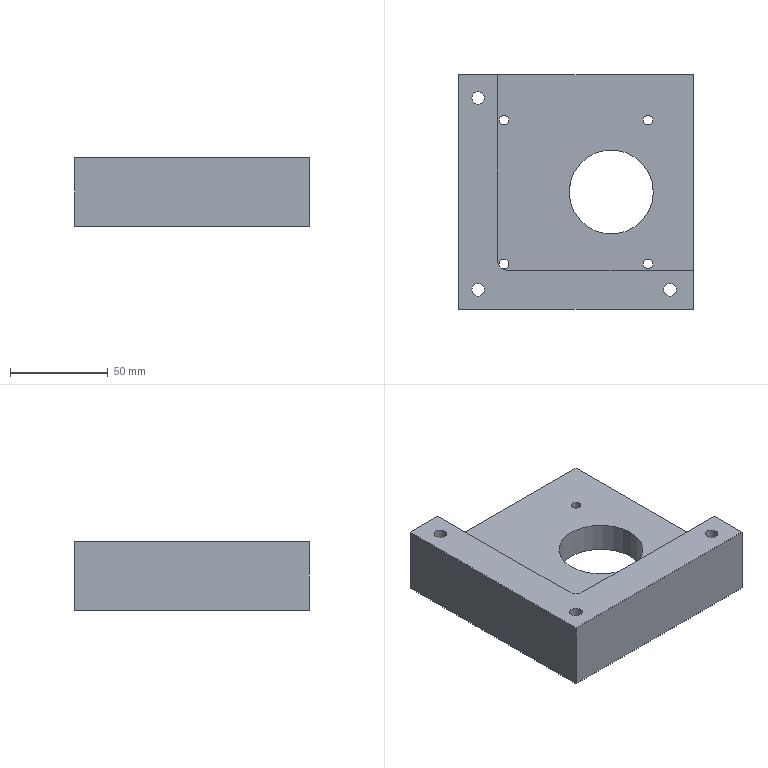Part | NX | 1 solid | 24 faces | box 120 x 120 x 35 mm | volume 274066 mm3 | plane 12 | cylinder 12 | commonest cylinder face diameters 5 x4 6.5 x3 12 x3 10 x1 43 x1
STEP:
#1=CARTESIAN_POINT('',(-60.,60.,-17.5));
#2=VERTEX_POINT('',#1);
#3=CARTESIAN_POINT('',(-60.,-60.,-17.5));
#4=VERTEX_POINT('',#3);
#5=CARTESIAN_POINT('',(-60.,60.,-17.5));
#6=DIRECTION('',(0.,-1.,0.));
#7=VECTOR('',#6,1.);
#8=LINE('',#5,#7);
#9=EDGE_CURVE('',#2,#4,#8,.T.);
#10=ORIENTED_EDGE('',*,*,#9,.F.);
#11=CARTESIAN_POINT('',(60.,60.,-17.5));
#12=VERTEX_POINT('',#11);
#13=CARTESIAN_POINT('',(60.,60.,-17.5));
#14=DIRECTION('',(-1.,0.,0.));
#15=VECTOR('',#14,1.);
#16=LINE('',#13,#15);
#17=EDGE_CURVE('',#12,#2,#16,.T.);
#18=ORIENTED_EDGE('',*,*,#17,.F.);
#19=CARTESIAN_POINT('',(60.,-60.,-17.5));
#20=VERTEX_POINT('',#19);
#21=CARTESIAN_POINT('',(60.,-60.,-17.5));
#22=DIRECTION('',(0.,1.,0.));
#23=VECTOR('',#22,1.);
#24=LINE('',#21,#23);
#25=EDGE_CURVE('',#20,#12,#24,.T.);
#26=ORIENTED_EDGE('',*,*,#25,.F.);
#27=CARTESIAN_POINT('',(-60.,-60.,-17.5));
#28=DIRECTION('',(1.,0.,0.));
#29=VECTOR('',#28,1.);
#30=LINE('',#27,#29);
#31=EDGE_CURVE('',#4,#20,#30,.T.);
#32=ORIENTED_EDGE('',*,*,#31,.F.);
#33=EDGE_LOOP('',(#10,#18,#26,#32));
#34=FACE_BOUND('',#33,.T.);
#35=CARTESIAN_POINT('',(-39.27,36.77,-17.5));
#36=VERTEX_POINT('',#35);
#37=CARTESIAN_POINT('',(-36.77,36.77,-17.5));
#38=DIRECTION('',(0.,0.,-1.));
#39=DIRECTION('',(-1.,0.,0.));
#40=AXIS2_PLACEMENT_3D('',#37,#38,#39);
#41=CIRCLE('',#40,2.5);
#42=EDGE_CURVE('',#36,#36,#41,.T.);
#43=ORIENTED_EDGE('',*,*,#42,.F.);
#44=EDGE_LOOP('',(#43));
#45=FACE_BOUND('',#44,.T.);
#46=CARTESIAN_POINT('',(-39.27,-36.77,-17.5));
#47=VERTEX_POINT('',#46);
#48=CARTESIAN_POINT('',(-36.77,-36.77,-17.5));
#49=DIRECTION('',(0.,0.,-1.));
#50=DIRECTION('',(-1.,0.,0.));
#51=AXIS2_PLACEMENT_3D('',#48,#49,#50);
#52=CIRCLE('',#51,2.5);
#53=EDGE_CURVE('',#47,#47,#52,.T.);
#54=ORIENTED_EDGE('',*,*,#53,.F.);
#55=EDGE_LOOP('',(#54));
#56=FACE_BOUND('',#55,.T.);
#57=CARTESIAN_POINT('',(34.27,-36.77,-17.5));
#58=VERTEX_POINT('',#57);
#59=CARTESIAN_POINT('',(36.77,-36.77,-17.5));
#60=DIRECTION('',(0.,0.,-1.));
#61=DIRECTION('',(-1.,0.,0.));
#62=AXIS2_PLACEMENT_3D('',#59,#60,#61);
#63=CIRCLE('',#62,2.5);
#64=EDGE_CURVE('',#58,#58,#63,.T.);
#65=ORIENTED_EDGE('',*,*,#64,.F.);
#66=EDGE_LOOP('',(#65));
#67=FACE_BOUND('',#66,.T.);
#68=CARTESIAN_POINT('',(34.27,36.77,-17.5));
#69=VERTEX_POINT('',#68);
#70=CARTESIAN_POINT('',(36.77,36.77,-17.5));
#71=DIRECTION('',(0.,0.,-1.));
#72=DIRECTION('',(-1.,0.,0.));
#73=AXIS2_PLACEMENT_3D('',#70,#71,#72);
#74=CIRCLE('',#73,2.5);
#75=EDGE_CURVE('',#69,#69,#74,.T.);
#76=ORIENTED_EDGE('',*,*,#75,.F.);
#77=EDGE_LOOP('',(#76));
#78=FACE_BOUND('',#77,.T.);
#79=CARTESIAN_POINT('',(-3.5,0.,-17.5));
#80=VERTEX_POINT('',#79);
#81=CARTESIAN_POINT('',(18.,0.,-17.5));
#82=DIRECTION('',(0.,0.,-1.));
#83=DIRECTION('',(-1.,0.,0.));
#84=AXIS2_PLACEMENT_3D('',#81,#82,#83);
#85=CIRCLE('',#84,21.5);
#86=EDGE_CURVE('',#80,#80,#85,.T.);
#87=ORIENTED_EDGE('',*,*,#86,.F.);
#88=EDGE_LOOP('',(#87));
#89=FACE_BOUND('',#88,.T.);
#90=CARTESIAN_POINT('',(-56.,48.,-17.5));
#91=VERTEX_POINT('',#90);
#92=CARTESIAN_POINT('',(-50.,48.,-17.5));
#93=DIRECTION('',(0.,0.,-1.));
#94=DIRECTION('',(-1.,0.,0.));
#95=AXIS2_PLACEMENT_3D('',#92,#93,#94);
#96=CIRCLE('',#95,6.);
#97=EDGE_CURVE('',#91,#91,#96,.T.);
#98=ORIENTED_EDGE('',*,*,#97,.F.);
#99=EDGE_LOOP('',(#98));
#100=FACE_BOUND('',#99,.T.);
#101=CARTESIAN_POINT('',(-56.,-50.,-17.5));
#102=VERTEX_POINT('',#101);
#103=CARTESIAN_POINT('',(-50.,-50.,-17.5));
#104=DIRECTION('',(0.,0.,-1.));
#105=DIRECTION('',(-1.,0.,0.));
#106=AXIS2_PLACEMENT_3D('',#103,#104,#105);
#107=CIRCLE('',#106,6.);
#108=EDGE_CURVE('',#102,#102,#107,.T.);
#109=ORIENTED_EDGE('',*,*,#108,.F.);
#110=EDGE_LOOP('',(#109));
#111=FACE_BOUND('',#110,.T.);
#112=CARTESIAN_POINT('',(42.,-50.,-17.5));
#113=VERTEX_POINT('',#112);
#114=CARTESIAN_POINT('',(48.,-50.,-17.5));
#115=DIRECTION('',(0.,0.,-1.));
#116=DIRECTION('',(-1.,0.,0.));
#117=AXIS2_PLACEMENT_3D('',#114,#115,#116);
#118=CIRCLE('',#117,6.);
#119=EDGE_CURVE('',#113,#113,#118,.T.);
#120=ORIENTED_EDGE('',*,*,#119,.F.);
#121=EDGE_LOOP('',(#120));
#122=FACE_BOUND('',#121,.T.);
#123=CARTESIAN_POINT('',(0.,0.,-17.5));
#124=DIRECTION('',(0.,0.,1.));
#125=DIRECTION('',(1.,0.,0.));
#126=AXIS2_PLACEMENT_3D('',#123,#124,#125);
#127=PLANE('',#126);
#128=ADVANCED_FACE('',(#34,#45,#56,#67,#78,#89,#100,#111,#122),#127,.F.);
#129=CARTESIAN_POINT('',(-40.,60.,17.5));
#130=VERTEX_POINT('',#129);
#131=CARTESIAN_POINT('',(-40.,-35.,17.5));
#132=VERTEX_POINT('',#131);
#133=CARTESIAN_POINT('',(-40.,60.,17.5));
#134=DIRECTION('',(0.,-1.,0.));
#135=VECTOR('',#134,1.);
#136=LINE('',#133,#135);
#137=EDGE_CURVE('',#130,#132,#136,.T.);
#138=ORIENTED_EDGE('',*,*,#137,.F.);
#139=CARTESIAN_POINT('',(-60.,60.,17.5));
#140=VERTEX_POINT('',#139);
#141=CARTESIAN_POINT('',(-40.,60.,17.5));
#142=DIRECTION('',(-1.,0.,0.));
#143=VECTOR('',#142,1.);
#144=LINE('',#141,#143);
#145=EDGE_CURVE('',#130,#140,#144,.T.);
#146=ORIENTED_EDGE('',*,*,#145,.T.);
#147=CARTESIAN_POINT('',(-60.,-60.,17.5));
#148=VERTEX_POINT('',#147);
#149=CARTESIAN_POINT('',(-60.,60.,17.5));
#150=DIRECTION('',(0.,-1.,0.));
#151=VECTOR('',#150,1.);
#152=LINE('',#149,#151);
#153=EDGE_CURVE('',#140,#148,#152,.T.);
#154=ORIENTED_EDGE('',*,*,#153,.T.);
#155=CARTESIAN_POINT('',(60.,-60.,17.5));
#156=VERTEX_POINT('',#155);
#157=CARTESIAN_POINT('',(-60.,-60.,17.5));
#158=DIRECTION('',(1.,0.,0.));
#159=VECTOR('',#158,1.);
#160=LINE('',#157,#159);
#161=EDGE_CURVE('',#148,#156,#160,.T.);
#162=ORIENTED_EDGE('',*,*,#161,.T.);
#163=CARTESIAN_POINT('',(60.,-40.,17.5));
#164=VERTEX_POINT('',#163);
#165=CARTESIAN_POINT('',(60.,-60.,17.5));
#166=DIRECTION('',(0.,1.,0.));
#167=VECTOR('',#166,1.);
#168=LINE('',#165,#167);
#169=EDGE_CURVE('',#156,#164,#168,.T.);
#170=ORIENTED_EDGE('',*,*,#169,.T.);
#171=CARTESIAN_POINT('',(-35.,-40.,17.5));
#172=VERTEX_POINT('',#171);
#173=CARTESIAN_POINT('',(60.,-40.,17.5));
#174=DIRECTION('',(-1.,0.,0.));
#175=VECTOR('',#174,1.);
#176=LINE('',#173,#175);
#177=EDGE_CURVE('',#164,#172,#176,.T.);
#178=ORIENTED_EDGE('',*,*,#177,.T.);
#179=CARTESIAN_POINT('',(-35.,-35.,17.5));
#180=DIRECTION('',(0.,0.,-1.));
#181=DIRECTION('',(0.,-1.,0.));
#182=AXIS2_PLACEMENT_3D('',#179,#180,#181);
#183=CIRCLE('',#182,5.);
#184=EDGE_CURVE('',#172,#132,#183,.T.);
#185=ORIENTED_EDGE('',*,*,#184,.T.);
#186=EDGE_LOOP('',(#138,#146,#154,#162,#170,#178,#185));
#187=FACE_BOUND('',#186,.T.);
#188=CARTESIAN_POINT('',(-53.25,-50.,17.5));
#189=VERTEX_POINT('',#188);
#190=CARTESIAN_POINT('',(-50.,-50.,17.5));
#191=DIRECTION('',(0.,0.,-1.));
#192=DIRECTION('',(-1.,0.,0.));
#193=AXIS2_PLACEMENT_3D('',#190,#191,#192);
#194=CIRCLE('',#193,3.25);
#195=EDGE_CURVE('',#189,#189,#194,.T.);
#196=ORIENTED_EDGE('',*,*,#195,.T.);
#197=EDGE_LOOP('',(#196));
#198=FACE_BOUND('',#197,.T.);
#199=CARTESIAN_POINT('',(-53.25,48.,17.5));
#200=VERTEX_POINT('',#199);
#201=CARTESIAN_POINT('',(-50.,48.,17.5));
#202=DIRECTION('',(0.,0.,-1.));
#203=DIRECTION('',(-1.,0.,0.));
#204=AXIS2_PLACEMENT_3D('',#201,#202,#203);
#205=CIRCLE('',#204,3.25);
#206=EDGE_CURVE('',#200,#200,#205,.T.);
#207=ORIENTED_EDGE('',*,*,#206,.T.);
#208=EDGE_LOOP('',(#207));
#209=FACE_BOUND('',#208,.T.);
#210=CARTESIAN_POINT('',(44.75,-50.,17.5));
#211=VERTEX_POINT('',#210);
#212=CARTESIAN_POINT('',(48.,-50.,17.5));
#213=DIRECTION('',(0.,0.,-1.));
#214=DIRECTION('',(-1.,0.,0.));
#215=AXIS2_PLACEMENT_3D('',#212,#213,#214);
#216=CIRCLE('',#215,3.25);
#217=EDGE_CURVE('',#211,#211,#216,.T.);
#218=ORIENTED_EDGE('',*,*,#217,.T.);
#219=EDGE_LOOP('',(#218));
#220=FACE_BOUND('',#219,.T.);
#221=CARTESIAN_POINT('',(0.,0.,17.5));
#222=DIRECTION('',(0.,0.,1.));
#223=DIRECTION('',(1.,0.,0.));
#224=AXIS2_PLACEMENT_3D('',#221,#222,#223);
#225=PLANE('',#224);
#226=ADVANCED_FACE('',(#187,#198,#209,#220),#225,.T.);
#227=ORIENTED_EDGE('',*,*,#9,.T.);
#228=CARTESIAN_POINT('',(-60.,-60.,-17.5));
#229=DIRECTION('',(0.,0.,1.));
#230=VECTOR('',#229,1.);
#231=LINE('',#228,#230);
#232=EDGE_CURVE('',#4,#148,#231,.T.);
#233=ORIENTED_EDGE('',*,*,#232,.T.);
#234=ORIENTED_EDGE('',*,*,#153,.F.);
#235=CARTESIAN_POINT('',(-60.,60.,-17.5));
#236=DIRECTION('',(0.,0.,1.));
#237=VECTOR('',#236,1.);
#238=LINE('',#235,#237);
#239=EDGE_CURVE('',#2,#140,#238,.T.);
#240=ORIENTED_EDGE('',*,*,#239,.F.);
#241=EDGE_LOOP('',(#227,#233,#234,#240));
#242=FACE_OUTER_BOUND('',#241,.T.);
#243=CARTESIAN_POINT('',(-60.,60.,-17.5));
#244=DIRECTION('',(-1.,0.,0.));
#245=DIRECTION('',(0.,0.,1.));
#246=AXIS2_PLACEMENT_3D('',#243,#244,#245);
#247=PLANE('',#246);
#248=ADVANCED_FACE('',(#242),#247,.T.);
#249=ORIENTED_EDGE('',*,*,#31,.T.);
#250=CARTESIAN_POINT('',(60.,-60.,-17.5));
#251=DIRECTION('',(0.,0.,1.));
#252=VECTOR('',#251,1.);
#253=LINE('',#250,#252);
#254=EDGE_CURVE('',#20,#156,#253,.T.);
#255=ORIENTED_EDGE('',*,*,#254,.T.);
#256=ORIENTED_EDGE('',*,*,#161,.F.);
#257=ORIENTED_EDGE('',*,*,#232,.F.);
#258=EDGE_LOOP('',(#249,#255,#256,#257));
#259=FACE_OUTER_BOUND('',#258,.T.);
#260=CARTESIAN_POINT('',(-60.,-60.,-17.5));
#261=DIRECTION('',(0.,-1.,0.));
#262=DIRECTION('',(0.,0.,-1.));
#263=AXIS2_PLACEMENT_3D('',#260,#261,#262);
#264=PLANE('',#263);
#265=ADVANCED_FACE('',(#259),#264,.T.);
#266=CARTESIAN_POINT('',(60.,60.,-2.5));
#267=VERTEX_POINT('',#266);
#268=CARTESIAN_POINT('',(60.,-40.,-2.5));
#269=VERTEX_POINT('',#268);
#270=CARTESIAN_POINT('',(60.,60.,-2.5));
#271=DIRECTION('',(0.,-1.,0.));
#272=VECTOR('',#271,1.);
#273=LINE('',#270,#272);
#274=EDGE_CURVE('',#267,#269,#273,.T.);
#275=ORIENTED_EDGE('',*,*,#274,.T.);
#276=CARTESIAN_POINT('',(60.,-40.,17.5));
#277=DIRECTION('',(0.,0.,-1.));
#278=VECTOR('',#277,1.);
#279=LINE('',#276,#278);
#280=EDGE_CURVE('',#164,#269,#279,.T.);
#281=ORIENTED_EDGE('',*,*,#280,.F.);
#282=ORIENTED_EDGE('',*,*,#169,.F.);
#283=ORIENTED_EDGE('',*,*,#254,.F.);
#284=ORIENTED_EDGE('',*,*,#25,.T.);
#285=CARTESIAN_POINT('',(60.,60.,-17.5));
#286=DIRECTION('',(0.,0.,1.));
#287=VECTOR('',#286,1.);
#288=LINE('',#285,#287);
#289=EDGE_CURVE('',#12,#267,#288,.T.);
#290=ORIENTED_EDGE('',*,*,#289,.T.);
#291=EDGE_LOOP('',(#275,#281,#282,#283,#284,#290));
#292=FACE_OUTER_BOUND('',#291,.T.);
#293=CARTESIAN_POINT('',(60.,-60.,-17.5));
#294=DIRECTION('',(1.,0.,0.));
#295=DIRECTION('',(0.,0.,-1.));
#296=AXIS2_PLACEMENT_3D('',#293,#294,#295);
#297=PLANE('',#296);
#298=ADVANCED_FACE('',(#292),#297,.T.);
#299=CARTESIAN_POINT('',(-40.,60.,-2.5));
#300=VERTEX_POINT('',#299);
#301=CARTESIAN_POINT('',(60.,60.,-2.5));
#302=DIRECTION('',(-1.,0.,0.));
#303=VECTOR('',#302,1.);
#304=LINE('',#301,#303);
#305=EDGE_CURVE('',#267,#300,#304,.T.);
#306=ORIENTED_EDGE('',*,*,#305,.F.);
#307=ORIENTED_EDGE('',*,*,#289,.F.);
#308=ORIENTED_EDGE('',*,*,#17,.T.);
#309=ORIENTED_EDGE('',*,*,#239,.T.);
#310=ORIENTED_EDGE('',*,*,#145,.F.);
#311=CARTESIAN_POINT('',(-40.,60.,17.5));
#312=DIRECTION('',(0.,0.,-1.));
#313=VECTOR('',#312,1.);
#314=LINE('',#311,#313);
#315=EDGE_CURVE('',#130,#300,#314,.T.);
#316=ORIENTED_EDGE('',*,*,#315,.T.);
#317=EDGE_LOOP('',(#306,#307,#308,#309,#310,#316));
#318=FACE_OUTER_BOUND('',#317,.T.);
#319=CARTESIAN_POINT('',(60.,60.,-17.5));
#320=DIRECTION('',(0.,1.,0.));
#321=DIRECTION('',(0.,0.,1.));
#322=AXIS2_PLACEMENT_3D('',#319,#320,#321);
#323=PLANE('',#322);
#324=ADVANCED_FACE('',(#318),#323,.T.);
#325=CARTESIAN_POINT('',(-38.646,-38.421,-2.5));
#326=VERTEX_POINT('',#325);
#327=CARTESIAN_POINT('',(-38.421,-38.646,-2.5));
#328=VERTEX_POINT('',#327);
#329=CARTESIAN_POINT('',(-36.77,-36.77,-2.5));
#330=DIRECTION('',(0.,0.,-1.));
#331=DIRECTION('',(-1.,0.,0.));
#332=AXIS2_PLACEMENT_3D('',#329,#330,#331);
#333=CIRCLE('',#332,2.5);
#334=EDGE_CURVE('',#326,#328,#333,.T.);
#335=ORIENTED_EDGE('',*,*,#334,.T.);
#336=CARTESIAN_POINT('',(-35.,-40.,-2.5));
#337=VERTEX_POINT('',#336);
#338=CARTESIAN_POINT('',(-35.,-35.,-2.5));
#339=DIRECTION('',(0.,0.,1.));
#340=DIRECTION('',(-0.6843,-0.7292,0.));
#341=AXIS2_PLACEMENT_3D('',#338,#339,#340);
#342=CIRCLE('',#341,5.);
#343=EDGE_CURVE('',#328,#337,#342,.T.);
#344=ORIENTED_EDGE('',*,*,#343,.T.);
#345=CARTESIAN_POINT('',(-35.,-40.,-2.5));
#346=DIRECTION('',(1.,0.,0.));
#347=VECTOR('',#346,1.);
#348=LINE('',#345,#347);
#349=EDGE_CURVE('',#337,#269,#348,.T.);
#350=ORIENTED_EDGE('',*,*,#349,.T.);
#351=ORIENTED_EDGE('',*,*,#274,.F.);
#352=ORIENTED_EDGE('',*,*,#305,.T.);
#353=CARTESIAN_POINT('',(-40.,-35.,-2.5));
#354=VERTEX_POINT('',#353);
#355=CARTESIAN_POINT('',(-40.,60.,-2.5));
#356=DIRECTION('',(0.,-1.,0.));
#357=VECTOR('',#356,1.);
#358=LINE('',#355,#357);
#359=EDGE_CURVE('',#300,#354,#358,.T.);
#360=ORIENTED_EDGE('',*,*,#359,.T.);
#361=CARTESIAN_POINT('',(-35.,-35.,-2.5));
#362=DIRECTION('',(0.,0.,1.));
#363=DIRECTION('',(-1.,0.,0.));
#364=AXIS2_PLACEMENT_3D('',#361,#362,#363);
#365=CIRCLE('',#364,5.);
#366=EDGE_CURVE('',#354,#326,#365,.T.);
#367=ORIENTED_EDGE('',*,*,#366,.T.);
#368=EDGE_LOOP('',(#335,#344,#350,#351,#352,#360,#367));
#369=FACE_BOUND('',#368,.T.);
#370=CARTESIAN_POINT('',(34.27,-36.77,-2.5));
#371=VERTEX_POINT('',#370);
#372=CARTESIAN_POINT('',(36.77,-36.77,-2.5));
#373=DIRECTION('',(0.,0.,-1.));
#374=DIRECTION('',(-1.,0.,0.));
#375=AXIS2_PLACEMENT_3D('',#372,#373,#374);
#376=CIRCLE('',#375,2.5);
#377=EDGE_CURVE('',#371,#371,#376,.T.);
#378=ORIENTED_EDGE('',*,*,#377,.T.);
#379=EDGE_LOOP('',(#378));
#380=FACE_BOUND('',#379,.T.);
#381=CARTESIAN_POINT('',(34.27,36.77,-2.5));
#382=VERTEX_POINT('',#381);
#383=CARTESIAN_POINT('',(36.77,36.77,-2.5));
#384=DIRECTION('',(0.,0.,-1.));
#385=DIRECTION('',(-1.,0.,0.));
#386=AXIS2_PLACEMENT_3D('',#383,#384,#385);
#387=CIRCLE('',#386,2.5);
#388=EDGE_CURVE('',#382,#382,#387,.T.);
#389=ORIENTED_EDGE('',*,*,#388,.T.);
#390=EDGE_LOOP('',(#389));
#391=FACE_BOUND('',#390,.T.);
#392=CARTESIAN_POINT('',(-3.5,0.,-2.5));
#393=VERTEX_POINT('',#392);
#394=CARTESIAN_POINT('',(18.,0.,-2.5));
#395=DIRECTION('',(0.,0.,-1.));
#396=DIRECTION('',(-1.,0.,0.));
#397=AXIS2_PLACEMENT_3D('',#394,#395,#396);
#398=CIRCLE('',#397,21.5);
#399=EDGE_CURVE('',#393,#393,#398,.T.);
#400=ORIENTED_EDGE('',*,*,#399,.T.);
#401=EDGE_LOOP('',(#400));
#402=FACE_BOUND('',#401,.T.);
#403=CARTESIAN_POINT('',(-39.27,36.77,-2.5));
#404=VERTEX_POINT('',#403);
#405=CARTESIAN_POINT('',(-36.77,36.77,-2.5));
#406=DIRECTION('',(0.,0.,-1.));
#407=DIRECTION('',(-1.,0.,0.));
#408=AXIS2_PLACEMENT_3D('',#405,#406,#407);
#409=CIRCLE('',#408,2.5);
#410=EDGE_CURVE('',#404,#404,#409,.T.);
#411=ORIENTED_EDGE('',*,*,#410,.T.);
#412=EDGE_LOOP('',(#411));
#413=FACE_BOUND('',#412,.T.);
#414=CARTESIAN_POINT('',(0.,0.,-2.5));
#415=DIRECTION('',(0.,0.,1.));
#416=DIRECTION('',(1.,0.,0.));
#417=AXIS2_PLACEMENT_3D('',#414,#415,#416);
#418=PLANE('',#417);
#419=ADVANCED_FACE('',(#369,#380,#391,#402,#413),#418,.T.);
#420=CARTESIAN_POINT('',(-40.,-35.,17.5));
#421=DIRECTION('',(0.,0.,-1.));
#422=VECTOR('',#421,1.);
#423=LINE('',#420,#422);
#424=EDGE_CURVE('',#132,#354,#423,.T.);
#425=ORIENTED_EDGE('',*,*,#424,.T.);
#426=ORIENTED_EDGE('',*,*,#359,.F.);
#427=ORIENTED_EDGE('',*,*,#315,.F.);
#428=ORIENTED_EDGE('',*,*,#137,.T.);
#429=EDGE_LOOP('',(#425,#426,#427,#428));
#430=FACE_OUTER_BOUND('',#429,.T.);
#431=CARTESIAN_POINT('',(-40.,60.,17.5));
#432=DIRECTION('',(-1.,0.,0.));
#433=DIRECTION('',(0.,0.,1.));
#434=AXIS2_PLACEMENT_3D('',#431,#432,#433);
#435=PLANE('',#434);
#436=ADVANCED_FACE('',(#430),#435,.F.);
#437=CARTESIAN_POINT('',(-35.,-40.,17.5));
#438=DIRECTION('',(0.,0.,-1.));
#439=VECTOR('',#438,1.);
#440=LINE('',#437,#439);
#441=EDGE_CURVE('',#172,#337,#440,.T.);
#442=ORIENTED_EDGE('',*,*,#441,.F.);
#443=ORIENTED_EDGE('',*,*,#177,.F.);
#444=ORIENTED_EDGE('',*,*,#280,.T.);
#445=ORIENTED_EDGE('',*,*,#349,.F.);
#446=EDGE_LOOP('',(#442,#443,#444,#445));
#447=FACE_OUTER_BOUND('',#446,.T.);
#448=CARTESIAN_POINT('',(-40.,-40.,17.5));
#449=DIRECTION('',(0.,-1.,0.));
#450=DIRECTION('',(0.,0.,-1.));
#451=AXIS2_PLACEMENT_3D('',#448,#449,#450);
#452=PLANE('',#451);
#453=ADVANCED_FACE('',(#447),#452,.F.);
#454=ORIENTED_EDGE('',*,*,#366,.F.);
#455=ORIENTED_EDGE('',*,*,#424,.F.);
#456=ORIENTED_EDGE('',*,*,#184,.F.);
#457=ORIENTED_EDGE('',*,*,#441,.T.);
#458=ORIENTED_EDGE('',*,*,#343,.F.);
#459=CARTESIAN_POINT('',(-38.535,-38.536,-2.5));
#460=VERTEX_POINT('',#459);
#461=CARTESIAN_POINT('',(-38.421,-38.646,-2.5));
#462=CARTESIAN_POINT('',(-38.46,-38.61,-2.5));
#463=CARTESIAN_POINT('',(-38.498,-38.573,-2.5));
#464=CARTESIAN_POINT('',(-38.535,-38.536,-2.5));
#465=B_SPLINE_CURVE_WITH_KNOTS('',3,(#461,#462,#463,#464),.UNSPECIFIED.,.F.,.F.,(4,4),(0.,1.),.UNSPECIFIED.);
#466=EDGE_CURVE('',#328,#460,#465,.T.);
#467=ORIENTED_EDGE('',*,*,#466,.T.);
#468=CARTESIAN_POINT('',(-38.535,-38.536,-2.5));
#469=CARTESIAN_POINT('',(-38.573,-38.498,-2.5));
#470=CARTESIAN_POINT('',(-38.61,-38.46,-2.5));
#471=CARTESIAN_POINT('',(-38.646,-38.421,-2.5));
#472=B_SPLINE_CURVE_WITH_KNOTS('',3,(#468,#469,#470,#471),.UNSPECIFIED.,.F.,.F.,(4,4),(0.,1.),.UNSPECIFIED.);
#473=EDGE_CURVE('',#460,#326,#472,.T.);
#474=ORIENTED_EDGE('',*,*,#473,.T.);
#475=EDGE_LOOP('',(#454,#455,#456,#457,#458,#467,#474));
#476=FACE_OUTER_BOUND('',#475,.T.);
#477=CARTESIAN_POINT('',(-35.,-35.,17.792));
#478=DIRECTION('',(0.,0.,-1.));
#479=DIRECTION('',(0.,-1.,0.));
#480=AXIS2_PLACEMENT_3D('',#477,#478,#479);
#481=CYLINDRICAL_SURFACE('',#480,5.);
#482=ADVANCED_FACE('',(#476),#481,.F.);
#483=ORIENTED_EDGE('',*,*,#42,.T.);
#484=EDGE_LOOP('',(#483));
#485=FACE_BOUND('',#484,.T.);
#486=ORIENTED_EDGE('',*,*,#410,.F.);
#487=EDGE_LOOP('',(#486));
#488=FACE_BOUND('',#487,.T.);
#489=CARTESIAN_POINT('',(-36.77,36.77,-17.5));
#490=DIRECTION('',(0.,0.,-1.));
#491=DIRECTION('',(-1.,0.,0.));
#492=AXIS2_PLACEMENT_3D('',#489,#490,#491);
#493=CYLINDRICAL_SURFACE('',#492,2.5);
#494=ADVANCED_FACE('',(#485,#488),#493,.F.);
#495=ORIENTED_EDGE('',*,*,#53,.T.);
#496=EDGE_LOOP('',(#495));
#497=FACE_BOUND('',#496,.T.);
#498=ORIENTED_EDGE('',*,*,#334,.F.);
#499=ORIENTED_EDGE('',*,*,#473,.F.);
#500=ORIENTED_EDGE('',*,*,#466,.F.);
#501=EDGE_LOOP('',(#498,#499,#500));
#502=FACE_BOUND('',#501,.T.);
#503=CARTESIAN_POINT('',(-36.77,-36.77,-17.5));
#504=DIRECTION('',(0.,0.,-1.));
#505=DIRECTION('',(-1.,0.,0.));
#506=AXIS2_PLACEMENT_3D('',#503,#504,#505);
#507=CYLINDRICAL_SURFACE('',#506,2.5);
#508=ADVANCED_FACE('',(#497,#502),#507,.F.);
#509=ORIENTED_EDGE('',*,*,#64,.T.);
#510=EDGE_LOOP('',(#509));
#511=FACE_BOUND('',#510,.T.);
#512=ORIENTED_EDGE('',*,*,#377,.F.);
#513=EDGE_LOOP('',(#512));
#514=FACE_BOUND('',#513,.T.);
#515=CARTESIAN_POINT('',(36.77,-36.77,-17.5));
#516=DIRECTION('',(0.,0.,-1.));
#517=DIRECTION('',(-1.,0.,0.));
#518=AXIS2_PLACEMENT_3D('',#515,#516,#517);
#519=CYLINDRICAL_SURFACE('',#518,2.5);
#520=ADVANCED_FACE('',(#511,#514),#519,.F.);
#521=ORIENTED_EDGE('',*,*,#75,.T.);
#522=EDGE_LOOP('',(#521));
#523=FACE_BOUND('',#522,.T.);
#524=ORIENTED_EDGE('',*,*,#388,.F.);
#525=EDGE_LOOP('',(#524));
#526=FACE_BOUND('',#525,.T.);
#527=CARTESIAN_POINT('',(36.77,36.77,-17.5));
#528=DIRECTION('',(0.,0.,-1.));
#529=DIRECTION('',(-1.,0.,0.));
#530=AXIS2_PLACEMENT_3D('',#527,#528,#529);
#531=CYLINDRICAL_SURFACE('',#530,2.5);
#532=ADVANCED_FACE('',(#523,#526),#531,.F.);
#533=ORIENTED_EDGE('',*,*,#86,.T.);
#534=EDGE_LOOP('',(#533));
#535=FACE_BOUND('',#534,.T.);
#536=ORIENTED_EDGE('',*,*,#399,.F.);
#537=EDGE_LOOP('',(#536));
#538=FACE_BOUND('',#537,.T.);
#539=CARTESIAN_POINT('',(18.,0.,-17.5));
#540=DIRECTION('',(0.,0.,-1.));
#541=DIRECTION('',(-1.,0.,0.));
#542=AXIS2_PLACEMENT_3D('',#539,#540,#541);
#543=CYLINDRICAL_SURFACE('',#542,21.5);
#544=ADVANCED_FACE('',(#535,#538),#543,.F.);
#545=CARTESIAN_POINT('',(-53.25,-50.,-2.5));
#546=VERTEX_POINT('',#545);
#547=CARTESIAN_POINT('',(-50.,-50.,-2.5));
#548=DIRECTION('',(0.,0.,-1.));
#549=DIRECTION('',(-1.,0.,0.));
#550=AXIS2_PLACEMENT_3D('',#547,#548,#549);
#551=CIRCLE('',#550,3.25);
#552=EDGE_CURVE('',#546,#546,#551,.T.);
#553=ORIENTED_EDGE('',*,*,#552,.T.);
#554=EDGE_LOOP('',(#553));
#555=FACE_BOUND('',#554,.T.);
#556=ORIENTED_EDGE('',*,*,#195,.F.);
#557=EDGE_LOOP('',(#556));
#558=FACE_BOUND('',#557,.T.);
#559=CARTESIAN_POINT('',(-50.,-50.,-17.5));
#560=DIRECTION('',(0.,0.,-1.));
#561=DIRECTION('',(-1.,0.,0.));
#562=AXIS2_PLACEMENT_3D('',#559,#560,#561);
#563=CYLINDRICAL_SURFACE('',#562,3.25);
#564=ADVANCED_FACE('',(#555,#558),#563,.F.);
#565=CARTESIAN_POINT('',(-53.25,48.,-2.5));
#566=VERTEX_POINT('',#565);
#567=CARTESIAN_POINT('',(-50.,48.,-2.5));
#568=DIRECTION('',(0.,0.,-1.));
#569=DIRECTION('',(-1.,0.,0.));
#570=AXIS2_PLACEMENT_3D('',#567,#568,#569);
#571=CIRCLE('',#570,3.25);
#572=EDGE_CURVE('',#566,#566,#571,.T.);
#573=ORIENTED_EDGE('',*,*,#572,.T.);
#574=EDGE_LOOP('',(#573));
#575=FACE_BOUND('',#574,.T.);
#576=ORIENTED_EDGE('',*,*,#206,.F.);
#577=EDGE_LOOP('',(#576));
#578=FACE_BOUND('',#577,.T.);
#579=CARTESIAN_POINT('',(-50.,48.,-17.5));
#580=DIRECTION('',(0.,0.,-1.));
#581=DIRECTION('',(-1.,0.,0.));
#582=AXIS2_PLACEMENT_3D('',#579,#580,#581);
#583=CYLINDRICAL_SURFACE('',#582,3.25);
#584=ADVANCED_FACE('',(#575,#578),#583,.F.);
#585=CARTESIAN_POINT('',(44.75,-50.,-2.5));
#586=VERTEX_POINT('',#585);
#587=CARTESIAN_POINT('',(48.,-50.,-2.5));
#588=DIRECTION('',(0.,0.,-1.));
#589=DIRECTION('',(-1.,0.,0.));
#590=AXIS2_PLACEMENT_3D('',#587,#588,#589);
#591=CIRCLE('',#590,3.25);
#592=EDGE_CURVE('',#586,#586,#591,.T.);
#593=ORIENTED_EDGE('',*,*,#592,.T.);
#594=EDGE_LOOP('',(#593));
#595=FACE_BOUND('',#594,.T.);
#596=ORIENTED_EDGE('',*,*,#217,.F.);
#597=EDGE_LOOP('',(#596));
#598=FACE_BOUND('',#597,.T.);
#599=CARTESIAN_POINT('',(48.,-50.,-17.5));
#600=DIRECTION('',(0.,0.,-1.));
#601=DIRECTION('',(-1.,0.,0.));
#602=AXIS2_PLACEMENT_3D('',#599,#600,#601);
#603=CYLINDRICAL_SURFACE('',#602,3.25);
#604=ADVANCED_FACE('',(#595,#598),#603,.F.);
#605=CARTESIAN_POINT('',(-56.,48.,-2.5));
#606=VERTEX_POINT('',#605);
#607=CARTESIAN_POINT('',(-50.,48.,-2.5));
#608=DIRECTION('',(0.,0.,-1.));
#609=DIRECTION('',(-1.,0.,0.));
#610=AXIS2_PLACEMENT_3D('',#607,#608,#609);
#611=CIRCLE('',#610,6.);
#612=EDGE_CURVE('',#606,#606,#611,.T.);
#613=ORIENTED_EDGE('',*,*,#612,.T.);
#614=EDGE_LOOP('',(#613));
#615=FACE_BOUND('',#614,.T.);
#616=ORIENTED_EDGE('',*,*,#572,.F.);
#617=EDGE_LOOP('',(#616));
#618=FACE_BOUND('',#617,.T.);
#619=CARTESIAN_POINT('',(0.,0.,-2.5));
#620=DIRECTION('',(0.,0.,-1.));
#621=DIRECTION('',(-1.,0.,0.));
#622=AXIS2_PLACEMENT_3D('',#619,#620,#621);
#623=PLANE('',#622);
#624=ADVANCED_FACE('',(#615,#618),#623,.T.);
#625=CARTESIAN_POINT('',(-56.,-50.,-2.5));
#626=VERTEX_POINT('',#625);
#627=CARTESIAN_POINT('',(-50.,-50.,-2.5));
#628=DIRECTION('',(0.,0.,-1.));
#629=DIRECTION('',(-1.,0.,0.));
#630=AXIS2_PLACEMENT_3D('',#627,#628,#629);
#631=CIRCLE('',#630,6.);
#632=EDGE_CURVE('',#626,#626,#631,.T.);
#633=ORIENTED_EDGE('',*,*,#632,.T.);
#634=EDGE_LOOP('',(#633));
#635=FACE_BOUND('',#634,.T.);
#636=ORIENTED_EDGE('',*,*,#552,.F.);
#637=EDGE_LOOP('',(#636));
#638=FACE_BOUND('',#637,.T.);
#639=CARTESIAN_POINT('',(0.,0.,-2.5));
#640=DIRECTION('',(0.,0.,-1.));
#641=DIRECTION('',(-1.,0.,0.));
#642=AXIS2_PLACEMENT_3D('',#639,#640,#641);
#643=PLANE('',#642);
#644=ADVANCED_FACE('',(#635,#638),#643,.T.);
#645=CARTESIAN_POINT('',(42.,-50.,-2.5));
#646=VERTEX_POINT('',#645);
#647=CARTESIAN_POINT('',(48.,-50.,-2.5));
#648=DIRECTION('',(0.,0.,-1.));
#649=DIRECTION('',(-1.,0.,0.));
#650=AXIS2_PLACEMENT_3D('',#647,#648,#649);
#651=CIRCLE('',#650,6.);
#652=EDGE_CURVE('',#646,#646,#651,.T.);
#653=ORIENTED_EDGE('',*,*,#652,.T.);
#654=EDGE_LOOP('',(#653));
#655=FACE_BOUND('',#654,.T.);
#656=ORIENTED_EDGE('',*,*,#592,.F.);
#657=EDGE_LOOP('',(#656));
#658=FACE_BOUND('',#657,.T.);
#659=CARTESIAN_POINT('',(0.,0.,-2.5));
#660=DIRECTION('',(0.,0.,-1.));
#661=DIRECTION('',(-1.,0.,0.));
#662=AXIS2_PLACEMENT_3D('',#659,#660,#661);
#663=PLANE('',#662);
#664=ADVANCED_FACE('',(#655,#658),#663,.T.);
#665=ORIENTED_EDGE('',*,*,#97,.T.);
#666=EDGE_LOOP('',(#665));
#667=FACE_BOUND('',#666,.T.);
#668=ORIENTED_EDGE('',*,*,#612,.F.);
#669=EDGE_LOOP('',(#668));
#670=FACE_BOUND('',#669,.T.);
#671=CARTESIAN_POINT('',(-50.,48.,-17.5));
#672=DIRECTION('',(0.,0.,-1.));
#673=DIRECTION('',(-1.,0.,0.));
#674=AXIS2_PLACEMENT_3D('',#671,#672,#673);
#675=CYLINDRICAL_SURFACE('',#674,6.);
#676=ADVANCED_FACE('',(#667,#670),#675,.F.);
#677=ORIENTED_EDGE('',*,*,#108,.T.);
#678=EDGE_LOOP('',(#677));
#679=FACE_BOUND('',#678,.T.);
#680=ORIENTED_EDGE('',*,*,#632,.F.);
#681=EDGE_LOOP('',(#680));
#682=FACE_BOUND('',#681,.T.);
#683=CARTESIAN_POINT('',(-50.,-50.,-17.5));
#684=DIRECTION('',(0.,0.,-1.));
#685=DIRECTION('',(-1.,0.,0.));
#686=AXIS2_PLACEMENT_3D('',#683,#684,#685);
#687=CYLINDRICAL_SURFACE('',#686,6.);
#688=ADVANCED_FACE('',(#679,#682),#687,.F.);
#689=ORIENTED_EDGE('',*,*,#119,.T.);
#690=EDGE_LOOP('',(#689));
#691=FACE_BOUND('',#690,.T.);
#692=ORIENTED_EDGE('',*,*,#652,.F.);
#693=EDGE_LOOP('',(#692));
#694=FACE_BOUND('',#693,.T.);
#695=CARTESIAN_POINT('',(48.,-50.,-17.5));
#696=DIRECTION('',(0.,0.,-1.));
#697=DIRECTION('',(-1.,0.,0.));
#698=AXIS2_PLACEMENT_3D('',#695,#696,#697);
#699=CYLINDRICAL_SURFACE('',#698,6.);
#700=ADVANCED_FACE('',(#691,#694),#699,.F.);
#701=CLOSED_SHELL('',(#128,#226,#248,#265,#298,#324,#419,#436,#453,#482,#494,#508,#520,#532,#544,#564,#584,#604,#624,#644,#664,#676,#688,#700));
#702=MANIFOLD_SOLID_BREP('',#701);
#703=(LENGTH_UNIT()NAMED_UNIT(*)SI_UNIT(.MILLI.,.METRE.));
#704=UNCERTAINTY_MEASURE_WITH_UNIT(LENGTH_MEASURE(0.0508),#703,'','');
#705=(NAMED_UNIT(*)PLANE_ANGLE_UNIT()SI_UNIT($,.RADIAN.));
#706=PLANE_ANGLE_MEASURE_WITH_UNIT(PLANE_ANGLE_MEASURE(0.01745),#705);
#707=DIMENSIONAL_EXPONENTS(0.,0.,0.,0.,0.,0.,0.);
#708=(CONVERSION_BASED_UNIT('DEGREE',#706)NAMED_UNIT(#707)PLANE_ANGLE_UNIT());
#709=(NAMED_UNIT(*)SI_UNIT($,.STERADIAN.)SOLID_ANGLE_UNIT());
#710=(GEOMETRIC_REPRESENTATION_CONTEXT(3)GLOBAL_UNCERTAINTY_ASSIGNED_CONTEXT((#704))GLOBAL_UNIT_ASSIGNED_CONTEXT((#703,#708,#709))REPRESENTATION_CONTEXT('',''));
#711=ADVANCED_BREP_SHAPE_REPRESENTATION('',(#702),#710);